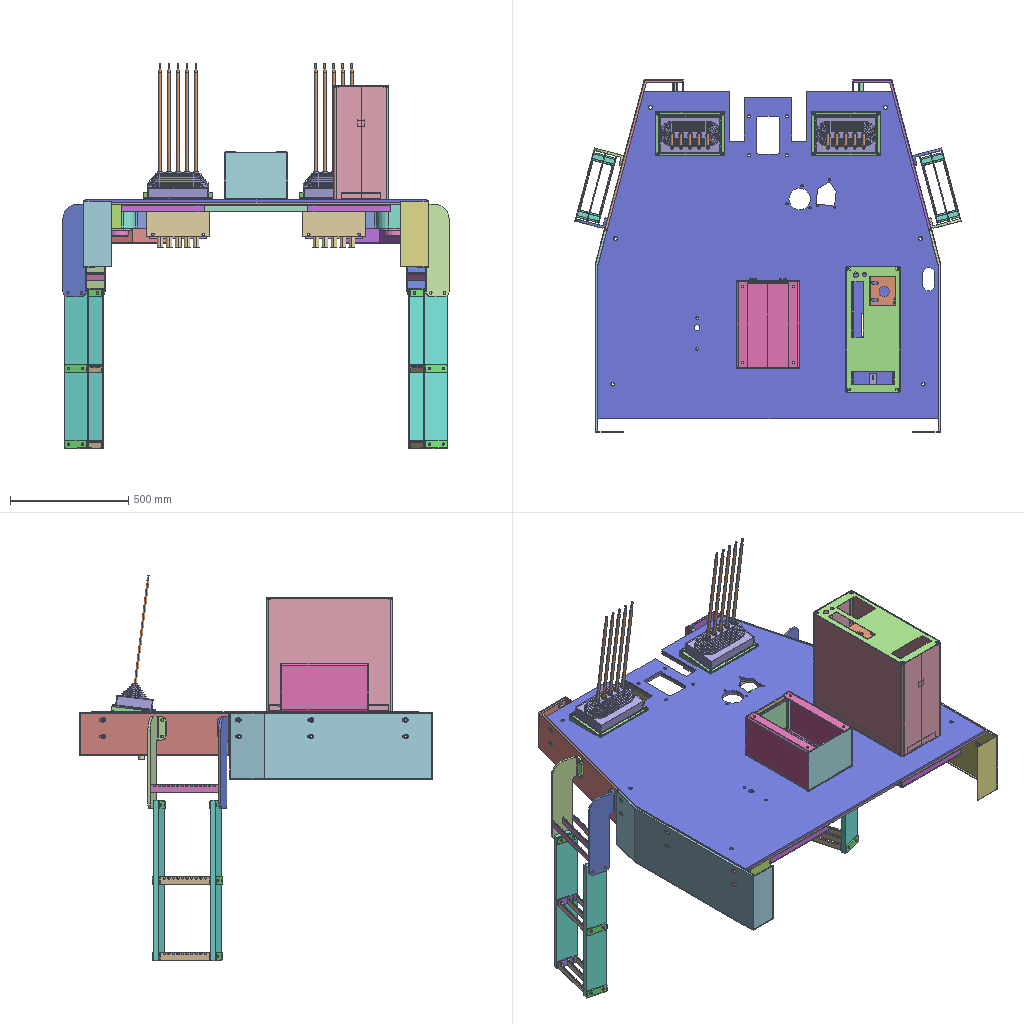Assembly | SolidWorks | 66 different items | 257 placed | box 1634 x 1493 x 1633 mm
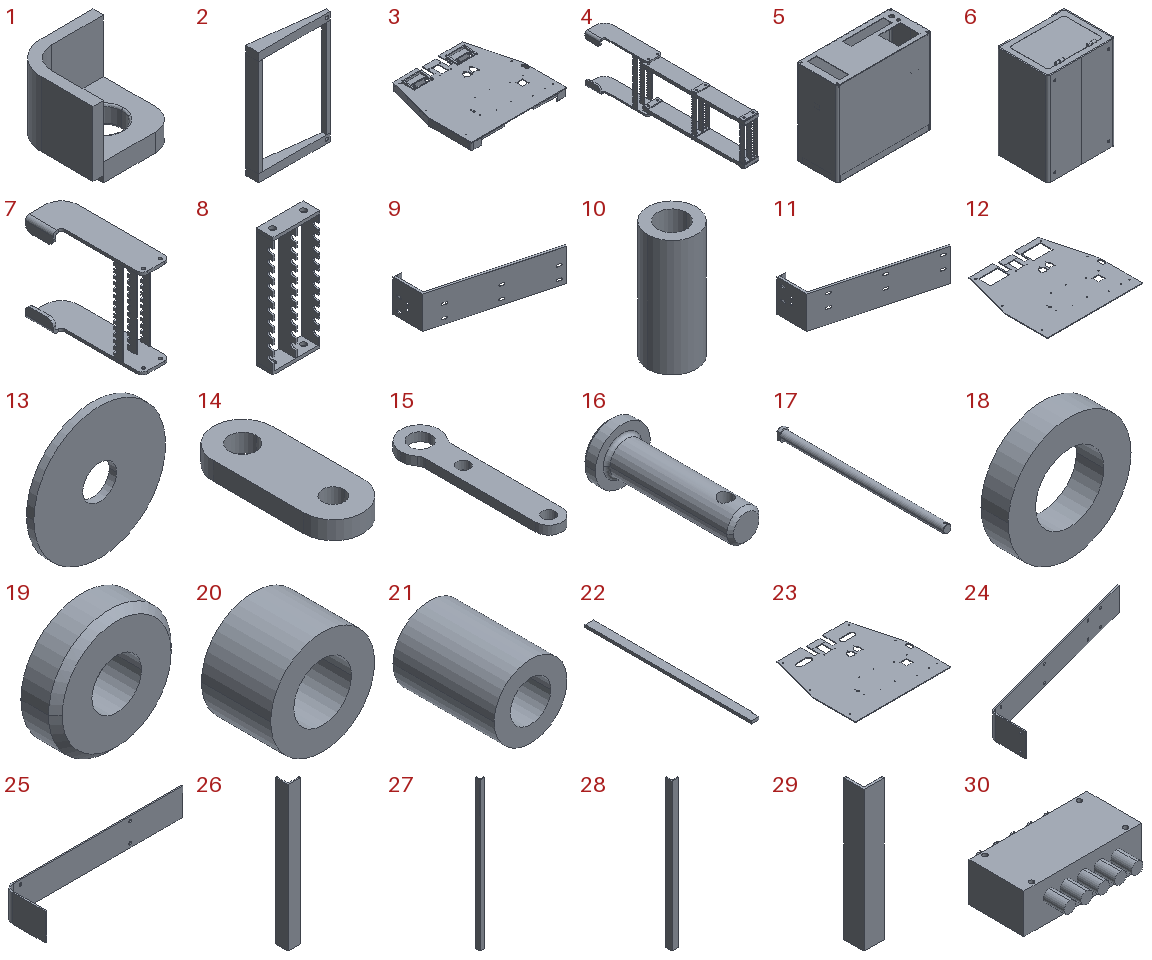Parts list (item | name | quantity | parent item | size | volume | features):
1 | (subassembly) | x6 | in 3 | 130 x 130 x 110 mm | 640650 mm3 | features RefAxis 1
2 | (subassembly) | x2 | in 3 | 184 x 32.592 x 290 mm | 260377 mm3 | -
3 | (subassembly) | x1 | - | 1440 x 1385 x 188.942 mm | 24430665 mm3 | -
4 | (subassembly) | x2 | - | 130 x 1035 x 320 mm | 3924769 mm3 | -
5 | (subassembly) | x1 | - | 536 x 231 x 482.5 mm | 2022797 mm3 | -
6 | (subassembly) | x1 | - | 270 x 206 x 382 mm | 1939837 mm3 | features RefAxis 2
7 | (subassembly) | x2 | in 4 | 130 x 390 x 320 mm | 950542 mm3 | -
8 | (subassembly) | x4 | in 4 | 90 x 32 x 230 mm | 87029 mm3 | -
9 | - | x1 | - | 635.787 x 334.526 x 180 mm | 341333 mm3 | features ICE 4, LPattern 3, BossThin 2, ExtruThin 1
10 | - | x4 | - | 20 x 20 x 48 mm | 9651 mm3 | features Extrusion 1
11 | - | x1 | - | 635.787 x 334.526 x 180 mm | 341333 mm3 | features ICE 4, LPattern 3, BossThin 2, ExtruThin 1
12 | - | x1 | - | 1440 x 1385 x 10 mm | 16649472 mm3 | features ICE 21, LPattern 10, Extrusion 1, Fillet 1
13 | - | x6 | - | 89 x 5 x 89 mm | 29028 mm3 | features Revolution 1
14 | - | x10 | - | 13 x 33 x 4 mm | 1385 mm3 | features Extrusion 1
15 | - | x20 | - | 18 x 75 x 4 mm | 3190 mm3 | features Extrusion 1
16 | - | x10 | - | 8 x 20 x 8 mm | 394.503 mm3 | features Chamfer 1, Fillet 1, ICE 1, Revolution 1
17 | - | x2 | - | 10 x 207 x 14 mm | 16414 mm3 | features ICE 3, Chamfer 1, Revolution 1
18 | - | x10 | - | 18 x 4 x 18 mm | 703.717 mm3 | features Revolution 1
19 | - | x6 | - | 89 x 25 x 89 mm | 126717 mm3 | features Chamfer 1, Revolution 1
20 | - | x4 | - | 18 x 12 x 18 mm | 2111 mm3 | features Revolution 1
21 | - | x8 | - | 18 x 25 x 18 mm | 4398 mm3 | features Revolution 1
22 | - | x1 | - | 30 x 610 x 10 mm | 182220 mm3 | features Extrusion 1, ICE 1
23 | - | x1 | in 3 | 1440 x 1385 x 10 mm | 17401314 mm3 | features ICE 21, LPattern 10, Extrusion 1, Fillet 1
24 | - | x2 | in 3 | 736.282 x 345 x 100 mm | 446241 mm3 | features ICE 3, LPattern 3, ExtruThin 1
25 | - | x2 | in 3 | 648 x 150 x 100 mm | 389028 mm3 | features ExtruThin 1, ICE 1, LPattern 1
26 | - | x2 | in 3 | 30 x 30 x 350 mm | 59550 mm3 | features Extrusion 1
27 | - | x1 | in 3 | 30 x 30 x 1024 mm | 174225 mm3 | features Extrusion 1
28 | - | x2 | in 3 | 30 x 30 x 692 mm | 117738 mm3 | features Extrusion 1
29 | - | x1 | in 3 | 30 x 30 x 210 mm | 35730 mm3 | features Extrusion 1
30 | - | x2 | - | 266 x 205.5 x 88.9 mm | 3043785 mm3 | features ICE 5, LPattern 4, Extrusion 1, RefAxis 1
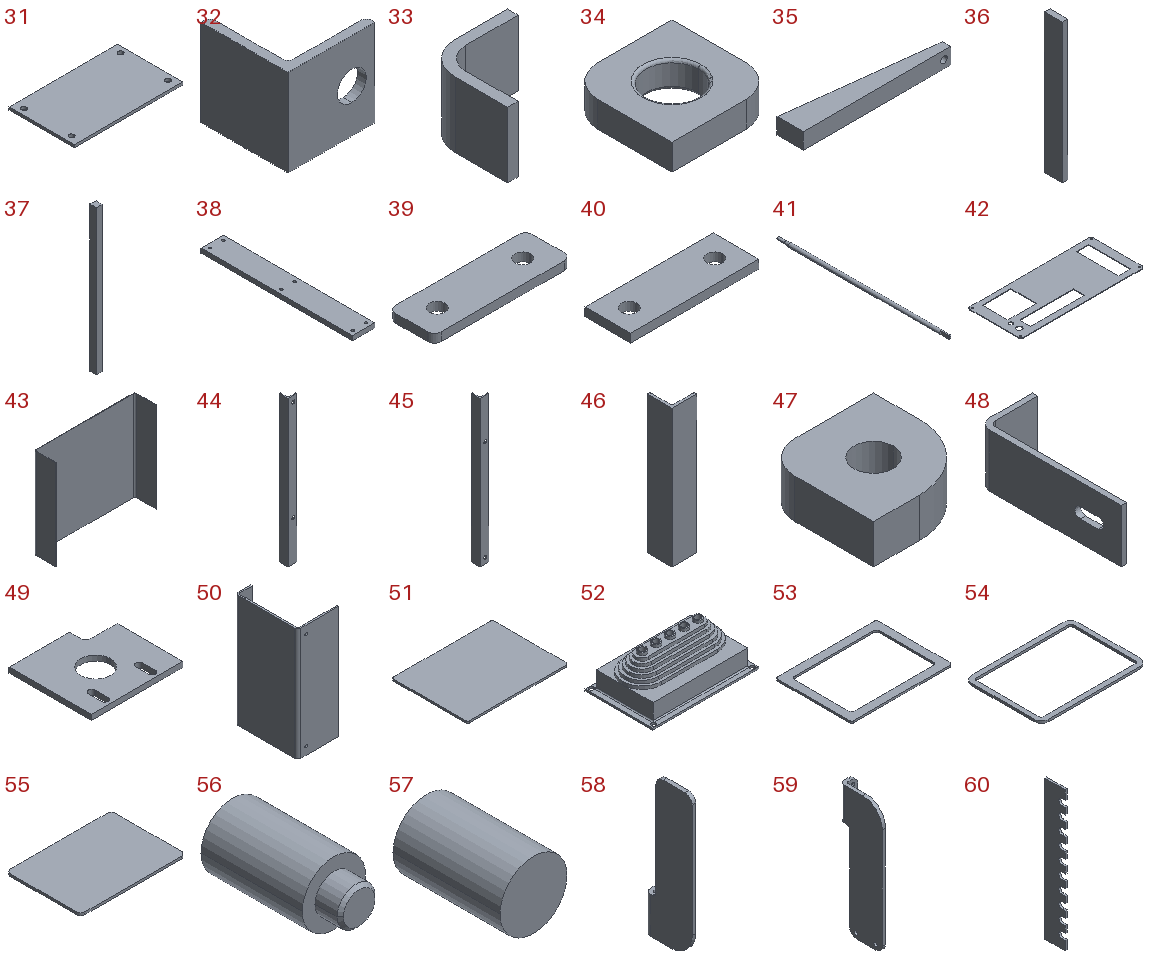31 | - | x2 | in 3 | 240 x 144 x 6 mm | 205079 mm3 | features Extrusion 1, ICE 1, LPattern 1, RefAxis 1
32 | - | x4 | in 3 | 30 x 30 x 30 mm | 4869 mm3 | features Extrusion 1, ICE 1
33 | - | x6 | in 1 | 130 x 130 x 100 mm | 361558 mm3 | features ExtruThin 1
34 | - | x6 | in 1 | 114 x 114 x 28 mm | 279092 mm3 | features Fillet 2, Extrusion 1
35 | - | x4 | in 2 | 184 x 32.592 x 20 mm | 77063 mm3 | features Extrusion 1, ICE 1, LPattern 1
36 | - | x2 | in 2 | 10 x 32.5 x 250 mm | 79715 mm3 | features Extrusion 1
37 | - | x2 | in 2 | 10 x 11.228 x 250 mm | 26535 mm3 | features Extrusion 1
38 | - | x4 | in 4 | 100 x 680 x 20 mm | 1348596 mm3 | features Extrusion 1, ICE 1, LPattern 1
39 | - | x12 | in 4 | 96 x 32 x 6 mm | 17163 mm3 | features Extrusion 1, Fillet 1, ICE 1, LPattern 1
40 | - | x8 | in 8 | 90 x 32 x 6 mm | 16140 mm3 | features Extrusion 1, ICE 1, LPattern 1
41 | - | x10 | - | 12 x 561 x 12 mm | 59373 mm3 | features ICE 3, Chamfer 1, RefAxis 1, Revolution 1
42 | - | x1 | in 5 | 535 x 230 x 2.5 mm | 217965 mm3 | features ICE 6, Extrusion 1, Fillet 1, LPattern 1
43 | - | x2 | in 5 | 536 x 115.5 x 480 mm | 725063 mm3 | features ExtruThin 1
44 | - | x1 | in 5 | 30 x 30 x 502 mm | 84841 mm3 | features Extrusion 1, ICE 1, LPattern 1
45 | - | x1 | in 5 | 30 x 30 x 502 mm | 84841 mm3 | features Extrusion 1, ICE 1, LPattern 1
46 | - | x2 | in 5 | 30 x 30 x 167 mm | 28414 mm3 | features Extrusion 1
47 | - | x4 | in 5 | 17 x 17 x 6 mm | 1403 mm3 | features Fillet 2, Extrusion 1, ICE 1
48 | - | x1 | in 5 | 30 x 80 x 30 mm | 9191 mm3 | features ExtruThin 1, ICE 1
49 | - | x1 | in 5 | 140 x 125 x 8 mm | 113392 mm3 | features ICE 3, Extrusion 1, Fillet 1, LPattern 1
50 | - | x2 | in 6 | 135 x 206 x 372 mm | 695413 mm3 | features ExtruThin 1, ICE 1, LPattern 1
51 | - | x1 | in 6 | 260 x 196 x 5 mm | 254693 mm3 | features Extrusion 1, Fillet 1
52 | - | x2 | - | 290 x 185 x 108 mm | 384373 mm3 | features ICE 18, BossThin 5, LPattern 3, RefAxis 2, Extrusion 1, Fillet 1
53 | - | x1 | in 6 | 260 x 196 x 5 mm | 83522 mm3 | features Fillet 2, Extrusion 1
54 | - | x1 | in 6 | 230 x 166 x 5 mm | 36742 mm3 | features Fillet 2, Extrusion 1
55 | - | x1 | in 6 | 219 x 155 x 5 mm | 169377 mm3 | features Extrusion 1, Fillet 1
56 | - | x2 | in 6 | 10 x 20 x 10 mm | 1368 mm3 | features Chamfer 1, Revolution 1
57 | - | x2 | in 6 | 10 x 16 x 10 mm | 971.407 mm3 | features Chamfer 1, ICE 1, Revolution 1
58 | - | x2 | in 7 | 45 x 130 x 390 mm | 437695 mm3 | features Fillet 3, ICE 3, LPattern 2, ExtruThin 1
59 | - | x2 | in 7 | 45 x 130 x 390 mm | 437695 mm3 | features Fillet 3, ICE 3, LPattern 2, ExtruThin 1
60 | - | x12 | in 8 | 3 x 32 x 218 mm | 18250 mm3 | features ExtruThin 1, ICE 1, LPattern 1
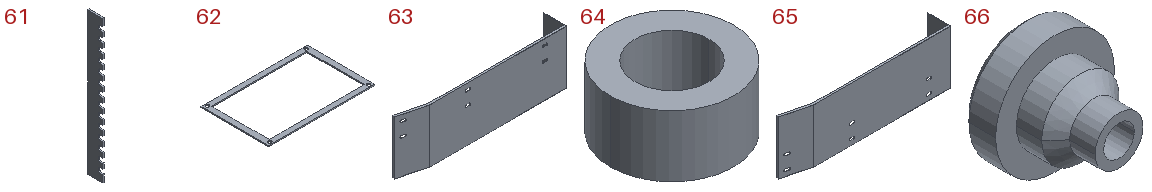61 | - | x6 | in 7 | 3 x 32 x 300 mm | 25051 mm3 | features ExtruThin 1, ICE 1, LPattern 1
62 | - | x2 | - | 290 x 185 x 3 mm | 37727 mm3 | features Extrusion 1, ICE 1, LPattern 1
63 | - | x1 | - | 856.99 x 120 x 280 mm | 584120 mm3 | features ICE 3, BossThin 2, LPattern 2, ExtruThin 1
64 | - | x24 | - | 20 x 20 x 10 mm | 2011 mm3 | features Extrusion 1
65 | - | x1 | - | 856.99 x 120 x 280 mm | 584120 mm3 | features ICE 3, BossThin 2, LPattern 2, ExtruThin 1
66 | - | x6 | - | 89 x 73 x 89 mm | 209040 mm3 | features Chamfer 1, Revolution 1
Mates (type | each side: item.copy, entity, surface, feature):
In the top assembly
Coincident | 23.1 face plane Boss-Extrude1 | 12.1 face plane Boss-Extrude1 | 3 times
Coincident | 34.1 face plane Boss-Extrude1 | 66.1 face plane Revolve1
Concentric | 34.1 face cylinder Boss-Extrude1 | 66.1 face cylinder Revolve1
Coincident | 34.2 face plane Boss-Extrude1 | 66.2 face plane Revolve1
Concentric | 34.2 face cylinder Boss-Extrude1 | 66.2 face cylinder Revolve1
Coincident | 34.3 face plane Boss-Extrude1 | 66.3 face plane Revolve1
Concentric | 34.3 face cylinder Boss-Extrude1 | 66.3 face cylinder Revolve1
Coincident | 34.4 face plane Boss-Extrude1 | 66.4 face plane Revolve1
Concentric | 34.4 face cylinder Boss-Extrude1 | 66.4 face cylinder Revolve1
Coincident | 34.5 face plane Boss-Extrude1 | 66.5 face plane Revolve1
Concentric | 34.5 face cylinder Boss-Extrude1 | 66.5 face cylinder Revolve1
Coincident | 34.6 face plane Boss-Extrude1 | 66.6 face plane Revolve1
Concentric | 34.6 face cylinder Boss-Extrude1 | 66.6 face cylinder Revolve1
Coincident | 34.6 face plane Boss-Extrude1 | 19.1 face plane Revolve1
Concentric | 66.6 face cylinder Revolve1 | 19.1 face cylinder Revolve1
Coincident | 34.5 face plane Boss-Extrude1 | 19.2 face plane Revolve1
Concentric | 66.5 face cylinder Revolve1 | 19.2 face cylinder Revolve1 | 2 times
Coincident | 34.4 face plane Boss-Extrude1 | 19.3 face plane Revolve1
Concentric | 66.4 face cylinder Revolve1 | 19.3 face cylinder Revolve1 | 2 times
Coincident | 34.1 face plane Boss-Extrude1 | 19.4 face plane Revolve1
Concentric | 66.1 face cylinder Revolve1 | 19.4 face cylinder Revolve1
Coincident | 34.2 face plane Boss-Extrude1 | 19.5 face plane Revolve1
Concentric | 66.2 face cylinder Revolve1 | 19.5 face cylinder Revolve1
Coincident | 34.3 face plane Boss-Extrude1 | 19.6 face plane Revolve1
Concentric | 66.3 face cylinder Revolve1 | 19.6 face cylinder Revolve1
Coincident | 66.1 face plane Revolve1 | 13.1 face plane Revolve1
Concentric | 66.1 face cylinder Revolve1 | 13.1 face cylinder Revolve1
Coincident | 66.2 face plane Revolve1 | 13.2 face plane Revolve1
Concentric | 66.2 face cylinder Revolve1 | 13.2 face cylinder Revolve1
Coincident | 66.6 face plane Revolve1 | 13.3 face plane Revolve1
Concentric | 66.6 face cylinder Revolve1 | 13.3 face cylinder Revolve1
Coincident | 66.5 face plane Revolve1 | 13.4 face plane Revolve1
Concentric | 66.5 face cylinder Revolve1 | 13.4 face cylinder Revolve1
Coincident | 66.3 face plane Revolve1 | 13.5 face plane Revolve1
Concentric | 66.3 face cylinder Revolve1 | 13.5 face cylinder Revolve1
Coincident | 66.4 face plane Revolve1 | 13.6 face plane Revolve1
Concentric | 66.4 face cylinder Revolve1 | 13.6 face cylinder Revolve1
Coincident | 31.1 face plane Boss-Extrude1 | 30.1 face plane Boss-Extrude1
Concentric | 31.1 face cylinder Cut-Extrude1 | 30.1 face cylinder LPattern1
Concentric | 31.1 face cylinder LPattern1 | 30.1 face cylinder LPattern1
Coincident | 31.2 face plane Boss-Extrude1 | 30.2 face plane Boss-Extrude1
Concentric | 31.2 face cylinder Cut-Extrude1 | 30.2 face cylinder LPattern1
Concentric | 31.2 face cylinder LPattern1 | 30.2 face cylinder LPattern1
Concentric | 32.1 face cylinder Cut-Extrude1 | 17.1 face cylinder Revolve1
Coincident | 32.1 face plane Boss-Extrude1 | 17.1 face plane Revolve1
Concentric | 32.2 face cylinder Cut-Extrude1 | 17.2 face cylinder Revolve1
Coincident | 32.3 face plane Boss-Extrude1 | 17.2 face plane Revolve1
Concentric | 30.2 face cylinder Cut-Extrude2 | 14.1 face cylinder Boss-Extrude1
Coincident | 30.2 face plane LPattern6 | 14.1 face plane Boss-Extrude1
Concentric | 14.1 face cylinder Boss-Extrude1 | 16.1 face cylinder Revolve1
DistanceDim | 16.1 face plane Revolve1 | 14.1 face plane Boss-Extrude1
Concentric | 17.1 face cylinder Revolve1 | 15.1 face cylinder Boss-Extrude1
Concentric | 14.1 face cylinder Boss-Extrude1 | 15.1 face cylinder Boss-Extrude1
Coincident | 14.1 face plane Boss-Extrude1 | 15.1 face plane Boss-Extrude1
Concentric | 17.1 face cylinder Revolve1 | 15.2 face cylinder Boss-Extrude1
Coincident | 14.1 face plane Boss-Extrude1 | 15.2 face plane Boss-Extrude1
Concentric | 15.1 face cylinder Boss-Extrude1 | 15.2 face cylinder Boss-Extrude1
Concentric | 17.1 face cylinder Revolve1 | 18.1 face cylinder Revolve1
Coincident | 15.1 face plane Boss-Extrude1 | 18.1 face plane Revolve1
Concentric | 17.1 face cylinder Revolve1 | 20.1 face cylinder Revolve1
Coincident | 15.1 face plane Boss-Extrude1 | 20.1 face plane Revolve1
Concentric | 17.1 face cylinder Revolve1 | 21.1 face cylinder Revolve1
Coincident | 15.2 face plane Boss-Extrude1 | 21.1 face plane Revolve1
Concentric | 30.2 face cylinder Cut-Extrude2 | 16.2 face cylinder Revolve1
DistanceDim | 16.2 face plane Revolve1 | 30.2 face plane LPattern6
Concentric | 14.2 face cylinder Boss-Extrude1 | 16.2 face cylinder Revolve1
Coincident | 30.2 face plane LPattern6 | 14.2 face plane Boss-Extrude1
Concentric | 17.1 face cylinder Revolve1 | 15.3 face cylinder Boss-Extrude1
Coincident | 14.2 face plane Boss-Extrude1 | 15.3 face plane Boss-Extrude1
Concentric | 14.2 face cylinder Boss-Extrude1 | 15.3 face cylinder Boss-Extrude1
Concentric | 17.1 face cylinder Revolve1 | 15.4 face cylinder Boss-Extrude1
Coincident | 14.2 face plane Boss-Extrude1 | 15.4 face plane Boss-Extrude1
Concentric | 15.3 face cylinder Boss-Extrude1 | 15.4 face cylinder Boss-Extrude1
Concentric | 17.1 face cylinder Revolve1 | 18.2 face cylinder Revolve1
Coincident | 15.4 face plane Boss-Extrude1 | 18.2 face plane Revolve1
Concentric | 17.1 face cylinder Revolve1 | 21.2 face cylinder Revolve1
Coincident | 15.3 face plane Boss-Extrude1 | 21.2 face plane Revolve1
Concentric | 30.2 face cylinder Cut-Extrude2 | 16.3 face cylinder Revolve1
DistanceDim | 16.3 face plane Revolve1 | 30.2 face plane LPattern6
Concentric | 14.3 face cylinder Boss-Extrude1 | 16.3 face cylinder Revolve1
Coincident | 30.2 face plane LPattern6 | 14.3 face plane Boss-Extrude1
Concentric | 17.1 face cylinder Revolve1 | 15.5 face cylinder Boss-Extrude1
Coincident | 14.3 face plane Boss-Extrude1 | 15.5 face plane Boss-Extrude1
Concentric | 14.3 face cylinder Boss-Extrude1 | 15.5 face cylinder Boss-Extrude1
Concentric | 17.1 face cylinder Revolve1 | 18.3 face cylinder Revolve1
Coincident | 15.5 face plane Boss-Extrude1 | 18.3 face plane Revolve1
Concentric | 17.1 face cylinder Revolve1 | 15.6 face cylinder Boss-Extrude1
Coincident | 14.3 face plane Boss-Extrude1 | 15.6 face plane Boss-Extrude1
Coincident | 14.3 edge | 15.6 face cylinder Boss-Extrude1
Concentric | 17.1 face cylinder Revolve1 | 21.3 face cylinder Revolve1
Coincident | 21.3 face plane Revolve1 | 15.6 face plane Boss-Extrude1
Concentric | 30.2 face cylinder Cut-Extrude2 | 16.4 face cylinder Revolve1
DistanceDim | 16.4 face plane Revolve1 | 30.2 face plane LPattern6
Concentric | 14.4 face cylinder Boss-Extrude1 | 16.4 face cylinder Revolve1
Coincident | 30.2 face plane LPattern6 | 14.4 face plane Boss-Extrude1
Concentric | 17.1 face cylinder Revolve1 | 15.7 face cylinder Boss-Extrude1
Coincident | 14.4 face plane Boss-Extrude1 | 15.7 face plane Boss-Extrude1
Concentric | 14.4 face cylinder Boss-Extrude1 | 15.7 face cylinder Boss-Extrude1
Concentric | 17.1 face cylinder Revolve1 | 15.8 face cylinder Boss-Extrude1
Coincident | 14.4 face plane Boss-Extrude1 | 15.8 face plane Boss-Extrude1
Concentric | 15.7 face cylinder Boss-Extrude1 | 15.8 face cylinder Boss-Extrude1
Concentric | 17.1 face cylinder Revolve1 | 18.4 face cylinder Revolve1
Coincident | 15.8 face plane Boss-Extrude1 | 18.4 face plane Revolve1
Concentric | 17.1 face cylinder Revolve1 | 21.4 face cylinder Revolve1
Coincident | 15.8 face plane Boss-Extrude1 | 21.4 face plane Revolve1
Concentric | 30.2 face cylinder Cut-Extrude2 | 16.5 face cylinder Revolve1
DistanceDim | 16.5 face plane Revolve1 | 30.2 face plane Cut-Extrude3
Concentric | 14.5 face cylinder Boss-Extrude1 | 16.5 face cylinder Revolve1
Coincident | 30.2 face plane Cut-Extrude3 | 14.5 face plane Boss-Extrude1
Coincident | 14.5 face plane Boss-Extrude1 | 15.9 face plane Boss-Extrude1
Concentric | 17.1 face cylinder Revolve1 | 15.9 face cylinder Boss-Extrude1
Concentric | 14.5 face cylinder Boss-Extrude1 | 15.9 face cylinder Boss-Extrude1
Concentric | 17.1 face cylinder Revolve1 | 15.10 face cylinder Boss-Extrude1
Coincident | 14.5 face plane Boss-Extrude1 | 15.10 face plane Boss-Extrude1
Concentric | 14.5 face cylinder Boss-Extrude1 | 15.10 face cylinder Boss-Extrude1
Coincident | 15.10 face plane Boss-Extrude1 | 18.5 face plane Revolve1
Concentric | 17.1 face cylinder Revolve1 | 18.5 face cylinder Revolve1
Coincident | 32.1 face plane Boss-Extrude1 | 20.2 face plane Revolve1
Concentric | 17.1 face cylinder Revolve1 | 20.2 face cylinder Revolve1
Concentric | 30.1 face cylinder Cut-Extrude2 | 16.6 face cylinder Revolve1
DistanceDim | 16.6 face plane Revolve1 | 30.1 face plane LPattern6
Coincident | 30.1 face plane LPattern6 | 14.6 face plane Boss-Extrude1
Concentric | 14.6 face cylinder Boss-Extrude1 | 16.6 face cylinder Revolve1
Coincident | 14.6 face plane Boss-Extrude1 | 15.11 face plane Boss-Extrude1
Concentric | 17.2 face cylinder Revolve1 | 15.11 face cylinder Boss-Extrude1
Concentric | 14.6 face cylinder Boss-Extrude1 | 15.11 face cylinder Boss-Extrude1
DistanceDim | 16.7 face plane Revolve1 | 16.6 face plane Revolve1
Concentric | 30.1 face cylinder Cut-Extrude2 | 16.7 face cylinder Revolve1
Coincident | 30.1 face plane LPattern6 | 14.7 face plane Boss-Extrude1
Concentric | 14.7 face cylinder Boss-Extrude1 | 16.7 face cylinder Revolve1
Coincident | 14.7 face plane Boss-Extrude1 | 15.12 face plane Boss-Extrude1
Concentric | 17.2 face cylinder Revolve1 | 15.12 face cylinder Boss-Extrude1
Concentric | 14.7 face cylinder Boss-Extrude1 | 15.12 face cylinder Boss-Extrude1
DistanceDim | 16.8 face plane Revolve1 | 16.7 face plane Revolve1
Concentric | 30.1 face cylinder Cut-Extrude2 | 16.8 face cylinder Revolve1
Coincident | 30.1 face plane LPattern6 | 14.8 face plane Boss-Extrude1
Concentric | 14.8 face cylinder Boss-Extrude1 | 16.8 face cylinder Revolve1
Coincident | 14.8 face plane Boss-Extrude1 | 15.13 face plane Boss-Extrude1
Concentric | 17.2 face cylinder Revolve1 | 15.13 face cylinder Boss-Extrude1
Concentric | 14.8 face cylinder Boss-Extrude1 | 15.13 face cylinder Boss-Extrude1
DistanceDim | 16.9 face plane Revolve1 | 16.8 face plane Revolve1
Concentric | 30.1 face cylinder Cut-Extrude2 | 16.9 face cylinder Revolve1
Coincident | 30.1 face plane LPattern6 | 14.9 face plane Boss-Extrude1
Concentric | 14.9 face cylinder Boss-Extrude1 | 16.9 face cylinder Revolve1
Coincident | 14.9 face plane Boss-Extrude1 | 15.14 face plane Boss-Extrude1
Concentric | 17.2 face cylinder Revolve1 | 15.14 face cylinder Boss-Extrude1
Concentric | 14.9 face cylinder Boss-Extrude1 | 15.14 face cylinder Boss-Extrude1
DistanceDim | 16.10 face plane Revolve1 | 16.9 face plane Revolve1
Concentric | 30.1 face cylinder Cut-Extrude2 | 16.10 face cylinder Revolve1
Coincident | 30.1 face plane Cut-Extrude3 | 14.10 face plane Boss-Extrude1
Concentric | 14.10 face cylinder Boss-Extrude1 | 16.10 face cylinder Revolve1
Coincident | 14.10 face plane Boss-Extrude1 | 15.15 face plane Boss-Extrude1
Concentric | 17.2 face cylinder Revolve1 | 15.15 face cylinder Boss-Extrude1
Concentric | 14.10 face cylinder Boss-Extrude1 | 15.15 face cylinder Boss-Extrude1
Coincident | 14.6 face plane Boss-Extrude1 | 15.16 face plane Boss-Extrude1
Concentric | 17.2 face cylinder Revolve1 | 15.16 face cylinder Boss-Extrude1
Concentric | 15.11 face cylinder Boss-Extrude1 | 15.16 face cylinder Boss-Extrude1
Coincident | 15.11 face plane Boss-Extrude1 | 18.6 face plane Revolve1
Concentric | 17.2 face cylinder Revolve1 | 18.6 face cylinder Revolve1
Coincident | 32.2 face plane Boss-Extrude1 | 20.3 face plane Revolve1
Concentric | 17.2 face cylinder Revolve1 | 20.3 face cylinder Revolve1
Coincident | 15.16 face plane Boss-Extrude1 | 21.5 face plane Revolve1
Concentric | 17.2 face cylinder Revolve1 | 21.5 face cylinder Revolve1
Coincident | 14.7 face plane Boss-Extrude1 | 15.17 face plane Boss-Extrude1
Concentric | 17.2 face cylinder Revolve1 | 15.17 face cylinder Boss-Extrude1
Concentric | 14.7 face cylinder Boss-Extrude1 | 15.17 face cylinder Boss-Extrude1
Coincident | 15.12 face plane Boss-Extrude1 | 18.7 face plane Revolve1
Concentric | 17.2 face cylinder Revolve1 | 18.7 face cylinder Revolve1
Coincident | 15.17 face plane Boss-Extrude1 | 21.6 face plane Revolve1
Concentric | 17.2 face cylinder Revolve1 | 21.6 face cylinder Revolve1
Coincident | 14.8 face plane Boss-Extrude1 | 15.18 face plane Boss-Extrude1
Concentric | 17.2 face cylinder Revolve1 | 15.18 face cylinder Boss-Extrude1
Concentric | 14.8 face cylinder Boss-Extrude1 | 15.18 face cylinder Boss-Extrude1
Concentric | 17.2 face cylinder Revolve1 | 20.4 face cylinder Revolve1
Coincident | 32.3 face plane Boss-Extrude1 | 20.4 face plane Revolve1
Coincident | 15.18 face plane Boss-Extrude1 | 21.7 face plane Revolve1
Concentric | 17.2 face cylinder Revolve1 | 21.7 face cylinder Revolve1
Coincident | 14.9 face plane Boss-Extrude1 | 15.19 face plane Boss-Extrude1
Concentric | 17.2 face cylinder Revolve1 | 15.19 face cylinder Boss-Extrude1
Concentric | 14.9 face cylinder Boss-Extrude1 | 15.19 face cylinder Boss-Extrude1
Coincident | 15.13 face plane Boss-Extrude1 | 18.8 face plane Revolve1
Concentric | 17.2 face cylinder Revolve1 | 18.8 face cylinder Revolve1
Coincident | 15.19 face plane Boss-Extrude1 | 21.8 face plane Revolve1
Concentric | 17.2 face cylinder Revolve1 | 21.8 face cylinder Revolve1
Coincident | 14.10 face plane Boss-Extrude1 | 15.20 face plane Boss-Extrude1
Concentric | 17.2 face cylinder Revolve1 | 15.20 face cylinder Boss-Extrude1
Concentric | 14.10 face cylinder Boss-Extrude1 | 15.20 face cylinder Boss-Extrude1
Coincident | 15.15 face plane Boss-Extrude1 | 18.9 face plane Revolve1
Concentric | 17.2 face cylinder Revolve1 | 18.9 face cylinder Revolve1
Coincident | 15.14 face plane Boss-Extrude1 | 18.10 face plane Revolve1
Concentric | 17.2 face cylinder Revolve1 | 18.10 face cylinder Revolve1
Coincident | 15.1 face plane Boss-Extrude1 | 41.1 face plane Cut-Extrude1
Concentric | 15.1 face cylinder Boss-Extrude1 | 41.1 face cylinder Cut-Extrude3
Parallel | 41.1 axis | assembly plane
Coincident | 15.4 face plane Boss-Extrude1 | 41.2 face plane Cut-Extrude1
Concentric | 15.4 face cylinder Boss-Extrude1 | 41.2 face cylinder Cut-Extrude3
Parallel | 41.1 axis | 41.2 axis
Coincident | 15.5 face plane Boss-Extrude1 | 41.3 face plane Cut-Extrude1
Coincident | 15.9 face plane Boss-Extrude1 | 41.4 face plane Cut-Extrude1
Concentric | 15.9 face cylinder Boss-Extrude1 | 41.4 face cylinder Cut-Extrude3
Concentric | 15.8 face cylinder Boss-Extrude1 | 41.3 face cylinder Cut-Extrude3
Coincident | 15.8 face plane Boss-Extrude1 | 41.5 face plane Cut-Extrude2
Concentric | 15.8 face cylinder Boss-Extrude1 | 41.5 face cylinder Cut-Extrude3
Parallel | 41.1 axis | 41.3 axis
Parallel | 41.1 axis | 41.5 axis
Parallel | 41.1 axis | 41.4 axis
Coincident | 15.11 face plane Boss-Extrude1 | 41.6 face plane Cut-Extrude1
Concentric | 15.16 face cylinder Boss-Extrude1 | 41.6 face cylinder Cut-Extrude3
Coincident | 15.17 face plane Boss-Extrude1 | 41.7 face plane Cut-Extrude2
Concentric | 15.17 face cylinder Boss-Extrude1 | 41.7 face cylinder Cut-Extrude3
Coincident | 15.13 face plane Boss-Extrude1 | 41.8 face plane Cut-Extrude1
Concentric | 15.13 face cylinder Boss-Extrude1 | 41.8 face cylinder Cut-Extrude3
Coincident | 15.14 face plane Boss-Extrude1 | 41.9 face plane Cut-Extrude1
Concentric | 15.14 face cylinder Boss-Extrude1 | 41.9 face cylinder Cut-Extrude3
Coincident | 15.15 face plane Boss-Extrude1 | 41.10 face plane Cut-Extrude1
Concentric | 15.15 face cylinder Boss-Extrude1 | 41.10 face cylinder Cut-Extrude3
Parallel | 41.1 axis | 41.6 axis
Parallel | 41.1 axis | 41.7 axis
Parallel | 41.1 axis | 41.8 axis
Parallel | 41.1 axis | 41.9 axis
Parallel | 41.1 axis | 41.10 axis
Coincident | 35.1 face plane Boss-Extrude1 | 52.1 face plane Boss-Extrude1 | 2 times
Concentric | 35.1 face cylinder Cut-Extrude1 | 52.1 face cylinder LPattern1
Coincident | 35.2 face plane Boss-Extrude1 | 52.2 face plane Boss-Extrude1 | 2 times
Concentric | 35.2 face cylinder Cut-Extrude1 | 52.2 face cylinder LPattern1
Coincident | 52.1 face plane Boss-Extrude1 | 62.1 face plane Boss-Extrude1 | 3 times
Coincident | 52.2 face plane Boss-Extrude1 | 62.2 face plane Boss-Extrude1 | 3 times
Coincident | 25.1 face plane Extrude-Thin1 | 64.1 face plane Boss-Extrude1
Concentric | 25.1 face cylinder Cut-Extrude1 | 64.1 face cylinder Boss-Extrude1
Coincident | 25.1 face plane Extrude-Thin1 | 64.2 face plane Boss-Extrude1
Concentric | 25.1 face cylinder LPattern1 | 64.2 face cylinder Boss-Extrude1
Coincident | 25.1 face plane Extrude-Thin1 | 64.3 face plane Boss-Extrude1
Concentric | 25.1 face cylinder LPattern1 | 64.3 face cylinder Boss-Extrude1
Coincident | 25.1 face plane Extrude-Thin1 | 64.4 face plane Boss-Extrude1
Concentric | 25.1 face cylinder LPattern1 | 64.4 face cylinder Boss-Extrude1
Coincident | 24.1 face plane Extrude-Thin1 | 64.5 face plane Boss-Extrude1
Concentric | 24.1 face cylinder LPattern1 | 64.5 face cylinder Boss-Extrude1
Coincident | 24.1 face plane Extrude-Thin1 | 64.6 face plane Boss-Extrude1
Concentric | 24.1 face cylinder Cut-Extrude1 | 64.6 face cylinder Boss-Extrude1
Coincident | 24.1 face plane Extrude-Thin1 | 64.7 face plane Boss-Extrude1
Concentric | 24.1 face cylinder Cut-Extrude2 | 64.7 face cylinder Boss-Extrude1
Coincident | 24.1 face plane Extrude-Thin1 | 64.8 face plane Boss-Extrude1
Concentric | 24.1 face cylinder LPattern2 | 64.8 face cylinder Boss-Extrude1
Coincident | 24.1 face plane Extrude-Thin1 | 64.9 face plane Boss-Extrude1
Concentric | 24.1 face cylinder LPattern2 | 64.9 face cylinder Boss-Extrude1
Coincident | 24.1 face plane Extrude-Thin1 | 64.10 face plane Boss-Extrude1
Concentric | 24.1 face cylinder LPattern2 | 64.10 face cylinder Boss-Extrude1
Coincident | 24.1 face plane Extrude-Thin1 | 64.11 face plane Boss-Extrude1
Concentric | 24.1 face cylinder LPattern2 | 64.11 face cylinder Boss-Extrude1
Coincident | 24.1 face plane Extrude-Thin1 | 64.12 face plane Boss-Extrude1
Concentric | 24.1 face cylinder LPattern2 | 64.12 face cylinder Boss-Extrude1
Coincident | 25.2 face plane Extrude-Thin1 | 64.13 face plane Boss-Extrude1
Concentric | 25.2 face cylinder LPattern1 | 64.13 face cylinder Boss-Extrude1
Coincident | 25.2 face plane Extrude-Thin1 | 64.14 face plane Boss-Extrude1
Concentric | 25.2 face cylinder Cut-Extrude1 | 64.14 face cylinder Boss-Extrude1
Coincident | 25.2 face plane Extrude-Thin1 | 64.15 face plane Boss-Extrude1
Concentric | 25.2 face cylinder LPattern1 | 64.15 face cylinder Boss-Extrude1
Coincident | 25.2 face plane Extrude-Thin1 | 64.16 face plane Boss-Extrude1
Concentric | 25.2 face cylinder LPattern1 | 64.16 face cylinder Boss-Extrude1
Coincident | 24.2 face plane Extrude-Thin1 | 64.17 face plane Boss-Extrude1
Concentric | 24.2 face cylinder Cut-Extrude1 | 64.17 face cylinder Boss-Extrude1
Coincident | 24.2 face plane Extrude-Thin1 | 64.18 face plane Boss-Extrude1
Concentric | 24.2 face cylinder LPattern1 | 64.18 face cylinder Boss-Extrude1
Coincident | 24.2 face plane Extrude-Thin1 | 64.19 face plane Boss-Extrude1
Concentric | 24.2 face cylinder Cut-Extrude2 | 64.19 face cylinder Boss-Extrude1
Coincident | 24.2 face plane Extrude-Thin1 | 64.20 face plane Boss-Extrude1
Concentric | 24.2 face cylinder LPattern2 | 64.20 face cylinder Boss-Extrude1
Coincident | 24.2 face plane Extrude-Thin1 | 64.21 face plane Boss-Extrude1
Concentric | 24.2 face cylinder LPattern2 | 64.21 face cylinder Boss-Extrude1
Coincident | 24.2 face plane Extrude-Thin1 | 64.22 face plane Boss-Extrude1
Concentric | 24.2 face cylinder LPattern2 | 64.22 face cylinder Boss-Extrude1
Coincident | 24.2 face plane Extrude-Thin1 | 64.23 face plane Boss-Extrude1
Concentric | 24.2 face cylinder LPattern2 | 64.23 face cylinder Boss-Extrude1
Coincident | 24.2 face plane Extrude-Thin1 | 64.24 face plane Boss-Extrude1
Concentric | 24.2 face cylinder LPattern2 | 64.24 face cylinder Boss-Extrude1
Coincident | 64.3 face plane Boss-Extrude1 | 63.1 face plane Extrude-Thin1
DistanceDim | 63.1 face plane Extrude-Thin2 | 12.1 face plane Boss-Extrude1
DistanceDim | 63.1 face plane Extrude-Thin1 | 23.1 face plane Boss-Extrude1
Coincident | 64.14 face plane Boss-Extrude1 | 65.1 face plane Extrude-Thin1
Coincident | 63.1 face plane Extrude-Thin2 | 65.1 face plane Extrude-Thin3
Coincident | 63.1 face plane Extrude-Thin1 | 65.1 face plane Extrude-Thin1
Coincident | 65.1 face plane Extrude-Thin3 | 9.1 face plane Extrude-Thin3
Coincident | 64.22 face plane Boss-Extrude1 | 9.1 face plane Extrude-Thin1
DistanceDim | 9.1 edge | 24.2 face plane Extrude-Thin1
Concentric | 24.2 face cylinder Cut-Extrude3 | 10.1 face cylinder Boss-Extrude1
Coincident | 24.2 face plane Extrude-Thin1 | 10.1 face plane Boss-Extrude1
Concentric | 24.2 face cylinder LPattern3 | 10.2 face cylinder Boss-Extrude1
Coincident | 24.2 face plane Extrude-Thin1 | 10.2 face plane Boss-Extrude1
Concentric | 24.1 face cylinder LPattern3 | 10.3 face cylinder Boss-Extrude1
Coincident | 24.1 face plane Extrude-Thin1 | 10.3 face plane Boss-Extrude1
Coincident | 24.1 face plane Extrude-Thin1 | 10.4 face plane Boss-Extrude1
Concentric | 24.1 face cylinder Cut-Extrude3 | 10.4 face cylinder Boss-Extrude1
Coincident | 64.9 face plane Boss-Extrude1 | 11.1 face plane Extrude-Thin1
Coincident | 63.1 face plane Extrude-Thin2 | 11.1 face plane Extrude-Thin2
DistanceDim | 11.1 edge | 24.1 face plane Extrude-Thin1
Coincident | 11.1 face plane Extrude-Thin1 | 59.1 face plane Extrude-Thin1
Concentric | 64.9 face cylinder Boss-Extrude1 | 59.1 face cylinder Cut-Extrude1
Concentric | 64.10 face cylinder Boss-Extrude1 | 59.1 face cylinder LPattern1
Coincident | 9.1 face plane Extrude-Thin1 | 59.2 face plane Extrude-Thin1
Concentric | 64.20 face cylinder Boss-Extrude1 | 59.2 face cylinder Cut-Extrude1
Concentric | 64.19 face cylinder Boss-Extrude1 | 59.2 face cylinder LPattern1
Coincident | 12.1 face plane Boss-Extrude1 | 45.1 face plane Boss-Extrude1
Concentric | 12.1 face cylinder LPattern4 | 45.1 face cylinder Cut-Extrude1
Concentric | 12.1 face cylinder Cut-Extrude6 | 45.1 face cylinder LPattern1
Coincident | 12.1 face plane Boss-Extrude1 | 50.1 face plane Extrude-Thin1
Concentric | 12.1 face cylinder LPattern5 | 50.1 face cylinder Cut-Extrude1
Concentric | 12.1 face cylinder Cut-Extrude7 | 50.2 face cylinder LPattern1
Symmetric | 12.1 face plane Boss-Extrude1 | 12.1 face plane Boss-Extrude1 | assembly plane
Coincident | 65.1 face plane Extrude-Thin1 | assembly plane
Coincident | 12.1 face plane Boss-Extrude1 | assembly plane
Coincident | 23.1 face plane Boss-Extrude1 | 22.1 face plane Boss-Extrude1
Coincident | 23.1 face plane Cut-Extrude20 | 22.1 face plane Boss-Extrude1
Coincident | 23.1 face plane Cut-Extrude21 | 22.1 face plane Boss-Extrude1
In subassembly 4
Coincident | 58.1 face plane Extrude-Thin1 | 38.1 face plane Boss-Extrude1
DistanceDim | 38.1 face plane Boss-Extrude1 | 58.1 face plane Extrude-Thin1
Concentric | 58.1 face cylinder LPattern2 | 38.1 face cylinder LPattern1
Coincident | 38.1 face plane Boss-Extrude1 | 38.2 face plane Boss-Extrude1 | 2 times
DistanceDim | 38.2 face plane Boss-Extrude1 | 59.3 face plane Extrude-Thin1
Coincident | 4.1 face | 39.1 face plane Boss-Extrude1
Concentric | 59.3 face cylinder LPattern2 | 39.1 face cylinder LPattern1
Coincident | 38.2 face plane Boss-Extrude1 | 39.1 face plane Boss-Extrude1
Coincident | 4.1 face | 39.2 face plane Boss-Extrude1
Coincident | 38.1 face plane Boss-Extrude1 | 39.2 face plane Boss-Extrude1
Concentric | 38.1 face cylinder LPattern1 | 39.2 face cylinder LPattern1
Coincident | 38.2 face plane Boss-Extrude1 | 39.3 face plane Boss-Extrude1
Concentric | 38.2 face cylinder LPattern1 | 39.3 face cylinder LPattern1
Coincident | 38.1 face plane Boss-Extrude1 | 39.4 face plane Boss-Extrude1
Concentric | 38.1 face cylinder LPattern1 | 39.4 face cylinder Cut-Extrude1
Coincident | 38.1 face plane Boss-Extrude1 | 39.5 face plane Boss-Extrude1
Concentric | 38.1 face cylinder LPattern1 | 39.5 face cylinder Cut-Extrude1
Coincident | 38.2 face plane Boss-Extrude1 | 39.6 face plane Boss-Extrude1
Concentric | 38.2 face cylinder LPattern1 | 39.6 face cylinder LPattern1
Concentric | 40.1 face cylinder LPattern1 | 39.4 face cylinder Cut-Extrude1
Concentric | 40.1 face cylinder Cut-Extrude1 | 39.4 face cylinder LPattern1
Coincident | 38.1 face plane Boss-Extrude1 | 40.1 face plane Boss-Extrude1
Concentric | 40.2 face cylinder LPattern1 | 39.5 face cylinder Cut-Extrude1
Concentric | 40.2 face cylinder Cut-Extrude1 | 39.5 face cylinder LPattern1
Coincident | 38.1 face plane Boss-Extrude1 | 40.2 face plane Boss-Extrude1
In subassembly 8
Coincident | 60.1 face plane Extrude-Thin1 | 40.3 face plane Boss-Extrude1 | 3 times
Coincident | 60.1 face plane Extrude-Thin1 | 40.4 face plane Boss-Extrude1 | 3 times
Coincident | 40.3 face plane Boss-Extrude1 | 60.2 face plane Extrude-Thin1
Coincident | 40.4 face plane Boss-Extrude1 | 60.2 face plane Extrude-Thin1 | 2 times
Coincident | 40.3 face plane Boss-Extrude1 | 60.3 face plane Extrude-Thin1 | 2 times
Width | 60.3 face plane Extrude-Thin1 | 60.3 face plane Extrude-Thin1 | 60.2 face plane Extrude-Thin1 | 60.1 face plane Extrude-Thin1
In subassembly 7
Coincident | 58.2 face plane Boss-Extrude1 | 59.4 face plane Boss-Extrude1
Coincident | 58.2 face plane Extrude-Thin1 | 59.4 face plane Extrude-Thin1
DistanceDim | 59.4 face plane Extrude-Thin1 | 58.2 face plane Extrude-Thin1
Coincident | 59.4 face plane Extrude-Thin1 | 61.1 face plane Extrude-Thin1 | 2 times
DistanceDim | 61.1 face plane Extrude-Thin1 | 59.4 face plane Boss-Extrude1
Coincident | 61.1 face plane Extrude-Thin1 | 61.2 face plane Extrude-Thin1
Coincident | 59.4 face plane Extrude-Thin1 | 61.2 face plane Extrude-Thin1
Coincident | 59.4 face plane Boss-Extrude1 | 61.2 face plane Extrude-Thin1
Coincident | 58.2 face plane Extrude-Thin1 | 61.3 face plane Extrude-Thin1
Width | 61.3 face plane Extrude-Thin1 | 61.3 face plane Extrude-Thin1 | 61.2 face plane Extrude-Thin1 | 61.1 face plane Extrude-Thin1
Coincident | 61.3 face plane Extrude-Thin1 | 61.2 face plane Extrude-Thin1
In subassembly 5
Coincident | 43.1 face plane Extrude-Thin1 | 43.2 face plane Extrude-Thin1 | 3 times
Coincident | 43.2 face plane Extrude-Thin1 | 45.2 face plane Boss-Extrude1 | 2 times
DistanceDim | 45.2 face plane Boss-Extrude1 | 43.2 face plane Extrude-Thin1
Coincident | 44.1 face plane Boss-Extrude1 | 45.2 face plane Boss-Extrude1 | 2 times
Coincident | 43.1 face plane Extrude-Thin1 | 44.1 face plane Boss-Extrude1
Coincident | 45.2 face plane Boss-Extrude1 | 46.1 face plane Boss-Extrude1
Coincident | 43.1 face plane Extrude-Thin1 | 46.1 face plane Boss-Extrude1
Coincident | 44.1 face plane Boss-Extrude1 | 46.1 face plane Boss-Extrude1
Coincident | 44.1 face plane Boss-Extrude1 | 46.2 face plane Boss-Extrude1
Coincident | 43.1 face plane Extrude-Thin1 | 46.2 face plane Boss-Extrude1
Coincident | 46.1 face plane Boss-Extrude1 | 46.2 face plane Boss-Extrude1
Coincident | 43.1 face plane Extrude-Thin1 | 47.1 face plane Boss-Extrude1 | 3 times
Coincident | 47.1 face plane Boss-Extrude1 | 47.2 face plane Boss-Extrude1
Coincident | 43.2 face plane Extrude-Thin1 | 47.2 face plane Boss-Extrude1 | 2 times
Coincident | 43.2 face plane Extrude-Thin1 | 47.3 face plane Boss-Extrude1 | 3 times
Coincident | 43.1 face plane Extrude-Thin1 | 47.4 face plane Boss-Extrude1 | 2 times
Coincident | 47.3 face plane Boss-Extrude1 | 47.4 face plane Boss-Extrude1
Coincident | 43.2 face plane Extrude-Thin1 | 49.1 face plane Boss-Extrude1
DistanceDim | 49.1 face plane Boss-Extrude1 | 43.2 face plane Extrude-Thin1
DistanceDim | 43.2 face plane Extrude-Thin1 | 49.1 face plane Boss-Extrude1
Coincident | 43.1 face plane Extrude-Thin1 | 48.1 face plane Extrude-Thin1
DistanceDim | 48.1 face plane Extrude-Thin1 | 43.1 face plane Extrude-Thin1
DistanceDim | 48.1 face plane Extrude-Thin1 | 43.2 face plane Extrude-Thin1
Coincident | 43.1 face plane Extrude-Thin1 | 42.1 face plane Boss-Extrude1
Concentric | 47.4 face cylinder Cut-Extrude1 | 42.1 face cylinder LPattern1
Concentric | 47.1 face cylinder Cut-Extrude1 | 42.1 face cylinder LPattern1
In subassembly 6
Coincident | 50.3 face plane Extrude-Thin1 | 50.4 face plane Extrude-Thin1 | 3 times
Coincident | 50.3 face plane Extrude-Thin1 | 51.1 face plane Boss-Extrude1
Coincident | 50.4 face plane Extrude-Thin1 | 51.1 face plane Boss-Extrude1 | 2 times
Coincident | 50.4 face plane Extrude-Thin1 | 53.1 face plane Boss-Extrude1 | 2 times
Coincident | 50.3 face plane Extrude-Thin1 | 53.1 face plane Boss-Extrude1
Coincident | 53.1 face plane Boss-Extrude1 | 54.1 face plane Boss-Extrude1
Width | 54.1 face plane Boss-Extrude1 | 54.1 face plane Boss-Extrude1 | 53.1 face plane Boss-Extrude1 | 53.1 face plane Boss-Extrude1 | 2 times
Width | 55.1 face plane Boss-Extrude1 | 55.1 face plane Boss-Extrude1 | 53.1 face plane Boss-Extrude1 | 53.1 face plane Boss-Extrude1 | 2 times
Coincident | 54.1 face plane Boss-Extrude1 | 55.1 face plane Boss-Extrude1
DistanceDim | 6.1 axis | 53.1 edge
Parallel | 53.1 edge | 6.1 axis
DistanceDim | 56.1 face plane Revolve1 | 53.1 face plane Boss-Extrude1
Coincident | 56.1 face plane Revolve1 | 57.1 face plane Revolve1
Concentric | 56.1 face cylinder Revolve1 | 57.1 face cylinder Revolve1
DistanceDim | 6.1 axis | 53.1 face plane Boss-Extrude1
DistanceDim | 56.2 face plane Revolve1 | 57.1 face plane Revolve1
Concentric | 57.1 face cylinder Revolve1 | 56.2 face cylinder Revolve1
Coincident | 56.2 face plane Revolve1 | 57.2 face plane Revolve1
Concentric | 56.2 face cylinder Revolve1 | 57.2 face cylinder Revolve1
In subassembly 3
Coincident | 23.2 face plane Boss-Extrude1 | 24.3 face plane Extrude-Thin1 | 3 times
Coincident | 23.2 face plane Boss-Extrude1 | 25.3 face plane Extrude-Thin1 | 3 times
Coincident | 23.2 face plane Boss-Extrude1 | 24.4 face plane Extrude-Thin1 | 3 times
Coincident | 23.2 face plane Boss-Extrude1 | 25.4 face plane Extrude-Thin1 | 3 times
Coincident | 23.2 face plane Boss-Extrude1 | 33.1 face plane Extrude-Thin1
DistanceDim | 33.1 face plane Extrude-Thin1 | 23.2 face plane Boss-Extrude1
DistanceDim | 1.1 axis | 23.2 plane
Coincident | 23.2 face plane Boss-Extrude1 | 33.2 face plane Extrude-Thin1
Coincident | 33.1 face plane Extrude-Thin1 | 33.2 face plane Extrude-Thin1
DistanceDim | 1.1 axis | 1.2 axis
Coincident | 23.2 face plane Boss-Extrude1 | 33.3 face plane Extrude-Thin1
DistanceDim | 33.1 face plane Extrude-Thin1 | 33.3 face plane Extrude-Thin1 | 2 times
Coincident | 23.2 face plane Boss-Extrude1 | 33.4 face plane Extrude-Thin1
Coincident | 33.3 face plane Extrude-Thin1 | 33.4 face plane Extrude-Thin1
DistanceDim | 33.3 face plane Extrude-Thin1 | 33.4 face plane Extrude-Thin1
Coincident | 23.2 face plane Boss-Extrude1 | 33.5 face plane Extrude-Thin1
DistanceDim | 33.5 face plane Extrude-Thin1 | 33.2 face plane Extrude-Thin1
Coincident | 33.3 face plane Extrude-Thin1 | 33.5 face plane Extrude-Thin1
Coincident | 23.2 face plane Boss-Extrude1 | 33.6 face plane Extrude-Thin1
Coincident | 33.5 face plane Extrude-Thin1 | 33.6 face plane Extrude-Thin1
Coincident | 33.4 face plane Extrude-Thin1 | 33.6 face plane Extrude-Thin1
Coincident | 23.2 face plane Boss-Extrude1 | 29.1 face plane Boss-Extrude1 | 2 times
Coincident | 24.4 face plane Extrude-Thin1 | 29.1 face plane Boss-Extrude1
Coincident | 33.1 face plane Extrude-Thin1 | 31.3 face plane Boss-Extrude1
Coincident | 1.1 axis | 31.3 plane
DistanceDim | 31.3 axis | 23.2 face plane Boss-Extrude1
Coincident | 33.2 face plane Extrude-Thin1 | 31.4 face plane Boss-Extrude1
Coincident | 31.3 face plane Boss-Extrude1 | 31.4 face plane Boss-Extrude1
Coincident | 1.2 axis | 31.4 plane
Coincident | 23.2 face plane Boss-Extrude1 | 35.3 face plane Boss-Extrude1
DistanceDim | 35.3 face plane Boss-Extrude1 | 31.4 plane
DistanceDim | 35.3 face plane Boss-Extrude1 | 23.2 face plane Cut-Extrude8
Coincident | 23.2 face plane Boss-Extrude1 | 35.4 face plane Boss-Extrude1
DistanceDim | 35.4 face plane Boss-Extrude1 | 31.3 plane
Coincident | 36.1 face plane Boss-Extrude1 | 36.2 face plane Boss-Extrude1
Coincident | 23.2 face plane Boss-Extrude1 | 32.4 face plane Boss-Extrude1
Coincident | 35.5 face plane Boss-Extrude1 | 32.4 face plane Boss-Extrude1
DistanceDim | 32.4 face plane Boss-Extrude1 | 23.2 face plane LPattern6
Coincident | 23.2 face plane Boss-Extrude1 | 32.5 face plane Boss-Extrude1
Coincident | 35.4 face plane Boss-Extrude1 | 32.5 face plane Boss-Extrude1
Coincident | 32.4 face plane Boss-Extrude1 | 32.5 face plane Boss-Extrude1
Coincident | 23.2 face plane Boss-Extrude1 | 32.6 face plane Boss-Extrude1
Coincident | 35.6 face plane Boss-Extrude1 | 32.6 face plane Boss-Extrude1
Coincident | 32.5 face plane Boss-Extrude1 | 32.6 face plane Boss-Extrude1
Coincident | 23.2 face plane Boss-Extrude1 | 32.7 face plane Boss-Extrude1
Coincident | 35.3 face plane Boss-Extrude1 | 32.7 face plane Boss-Extrude1
Coincident | 32.6 face plane Boss-Extrude1 | 32.7 face plane Boss-Extrude1
Coincident | 23.2 face plane Boss-Extrude1 | 26.1 face plane Boss-Extrude1
Coincident | 25.4 face plane Extrude-Thin1 | 26.1 face plane Boss-Extrude1 | 2 times
Coincident | 23.2 face plane Boss-Extrude1 | 27.1 face plane Boss-Extrude1
DistanceDim | 27.1 face plane Boss-Extrude1 | 26.1 face plane Boss-Extrude1
Coincident | 33.5 face plane Extrude-Thin1 | 27.1 face plane Boss-Extrude1
Coincident | 23.2 face plane Boss-Extrude1 | 28.1 face plane Boss-Extrude1
Coincident | 27.1 face plane Boss-Extrude1 | 28.1 face plane Boss-Extrude1
DistanceDim | 28.1 face plane Boss-Extrude1 | 25.4 face plane Extrude-Thin1
Coincident | 23.2 face plane Boss-Extrude1 | 28.2 face plane Boss-Extrude1
Coincident | 27.1 face plane Boss-Extrude1 | 28.2 face plane Boss-Extrude1
DistanceDim | 28.2 face plane Boss-Extrude1 | 25.3 face plane Extrude-Thin1
Coincident | 23.2 face plane Boss-Extrude1 | 26.2 face plane Boss-Extrude1 | 2 times
Coincident | 25.3 face plane Extrude-Thin1 | 26.2 face plane Boss-Extrude1
In subassembly 1
Coincident | 34.7 face plane Boss-Extrude1 | 33.7 face plane Extrude-Thin1 | 2 times
DistanceDim | 33.7 face plane Extrude-Thin1 | 34.7 face plane Boss-Extrude1
In subassembly 2
DistanceDim | 35.7 face plane Boss-Extrude1 | 35.8 face plane Boss-Extrude1
Coincident | 35.7 face plane Boss-Extrude1 | 35.8 face plane Boss-Extrude1 | 2 times
Coincident | 35.8 face plane Boss-Extrude1 | 36.3 face plane Boss-Extrude1 | 3 times
Coincident | 35.8 face plane Boss-Extrude1 | 37.1 face plane Boss-Extrude1 | 3 times